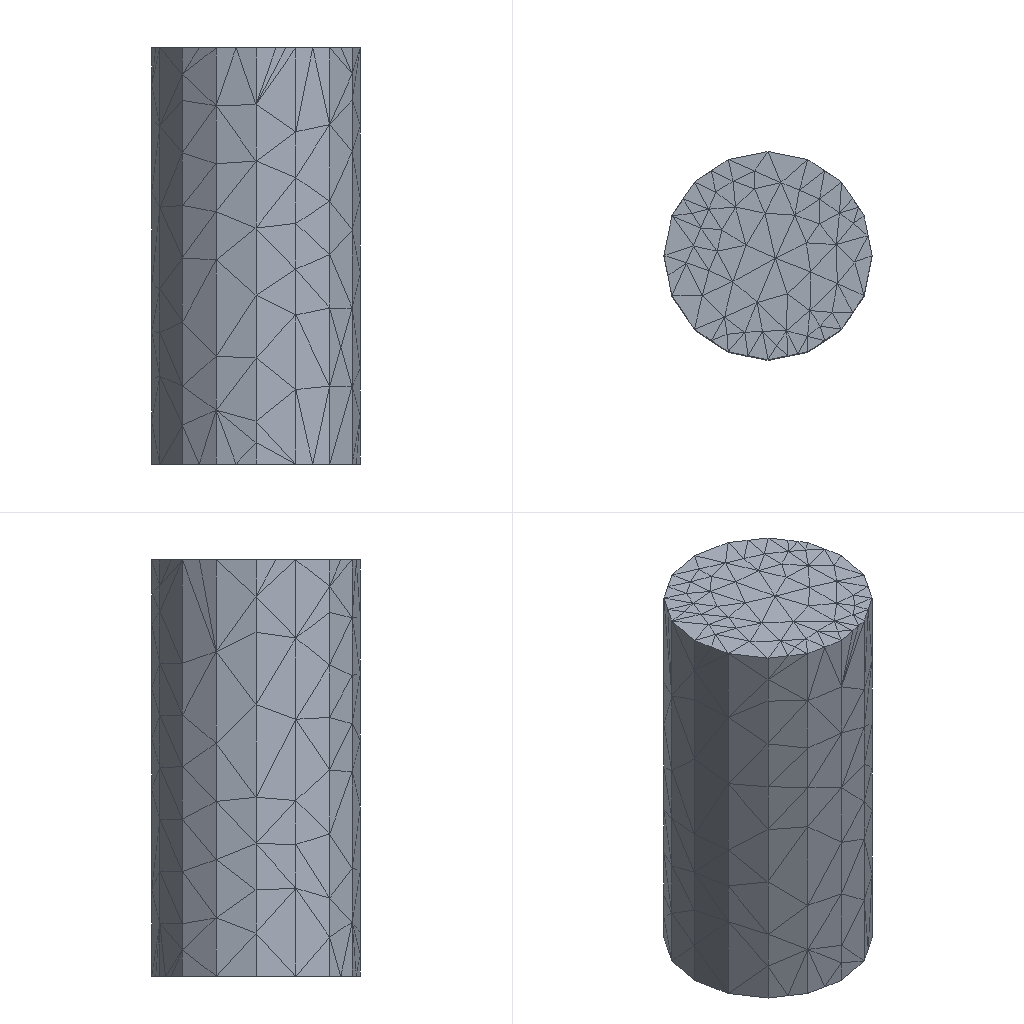Simulation study | ansys electronics desktop
Set-up summary:
category,name,step,type,value,unit,region
solver,ansys_electronics_desktop
units,length mm,,stated,model units
analysis,DESIGN_1,,HFSS Modal Network,design_type=HFSS
setup,Setup1,DESIGN_1,HfssDriven,frequency=10GHz; max_passes=6; max_delta_s=0.02
sweep,Sweep1,Setup1,Discrete,8GHz..12GHz n=9 step=
mesh,nodes,,,n/a (no mesh stored)
mesh,elements,,,n/a (no mesh stored)
material,vacuum,,permittivity,1
load,1,DESIGN_1,wave port,,,faces 8
load,2,DESIGN_1,wave port,,,faces 9
bc,PerfE,DESIGN_1,perfect e,,,faces 7
Ansys Electronics Desktop project file, long lists of numbers shortened, first 430 of 1282 lines:
$begin 'AnsoftProject'
	Created='Fri Sep  4 17:10:25 2026'
	Product='ElectronicsDesktop'
	FileOwnedByWorkbench=false
	$begin 'Desktop'
		Version(2026, 1)
		InfrastructureVersion(1, 0)
		$begin 'FactoryHeader'
			$begin 'geometry3deditor'
				KernelVersion(2, 0)
				ProjectContainsGeometry3D='1'
			$end 'geometry3deditor'
		$end 'FactoryHeader'
	$end 'Desktop'
	UsesAdvancedFeatures=false
	PreviewImageDesignId=1
	NextUniqueID=0
	MoveBackwards=false
	$begin 'HFSSEnvironment'
		Version(1, 0)
	$end 'HFSSEnvironment'
	$begin 'PlanarEMEnvironment'
		Version(1, 0)
	$end 'PlanarEMEnvironment'
	$begin 'Q3DEnvironment'
		Version(1, 0)
	$end 'Q3DEnvironment'
	$begin '2DExtractorEnvironment'
		Version(1, 0)
	$end '2DExtractorEnvironment'
	$begin 'NexximEnvironment'
		Version(1, 0)
	$end 'NexximEnvironment'
	$begin 'NexximNetlistEnvironment'
		Version(1, 0)
	$end 'NexximNetlistEnvironment'
	$begin 'EmitEnvironment'
		Version(1, 0)
	$end 'EmitEnvironment'
	$begin 'Maxwell3DEnvironment'
		Version(1, 0)
	$end 'Maxwell3DEnvironment'
	$begin 'Maxwell2DEnvironment'
		Version(1, 0)
	$end 'Maxwell2DEnvironment'
	$begin 'RMxprtEnvironment'
		Version(1, 0)
	$end 'RMxprtEnvironment'
	$begin 'MaxCirEnvironment'
		Version(1, 0)
	$end 'MaxCirEnvironment'
	$begin 'SimplorerEnvironment'
		Version(1, 0)
	$end 'SimplorerEnvironment'
	$begin 'IcepakEnvironment'
		Version(1, 0)
	$end 'IcepakEnvironment'
	$begin 'IcepakFEAEnvironment'
		Version(1, 0)
	$end 'IcepakFEAEnvironment'
	$begin 'SchematicEnvironment'
		Version(1, 0)
	$end 'SchematicEnvironment'
	$begin 'geometry3deditor'
		Version(1, 0)
	$end 'geometry3deditor'
	ReadVersion=12
	$begin 'DesignMgrEnvironment'
		CompInstCounter=1
		GPortCounter=0
		NetCounter=0
		Alias('Ieee;Simplorer Elements\\Ieee', 'Std;Simplorer Elements\\Std', 'Basic_VHDLAMS;Simplorer Elements\\Basic Elements VHDLAMS\\Basic Elements VHDLAMS', 'Digital_Elements;Simplorer Elements\\Digital Elements\\Digital Elements', 'Transformations;Simplorer Elements\\Tools\\Transformations\\Transformations', 'HEV_VHDLAMS;Simplorer Elements\\HEV VHDLAMS\\HEV VHDLAMS', 'automotive_vda;Simplorer Elem
	$end 'DesignMgrEnvironment'
	$begin 'ProjectDatasets'
		NextUniqueID=0
		MoveBackwards=false
		DatasetType='ProjectDatasetType'
		$begin 'DatasetDefinitions'
		$end 'DatasetDefinitions'
	$end 'ProjectDatasets'
	VariableOrders[0:]
	$begin 'Definitions'
		$begin 'Materials'
			$begin 'vacuum'
				CoordinateSystemType='Cartesian'
				BulkOrSurfaceType=1
				$begin 'PhysicsTypes'
					set('Electromagnetic')
				$end 'PhysicsTypes'
				$begin 'AttachedData'
					$begin 'MatAppearanceData'
						property_data='appearance_data'
						Red=230
						Green=230
						Blue=230
						Transparency=0.95
					$end 'MatAppearanceData'
				$end 'AttachedData'
				permittivity='1'
				ModTime=1499970477
				Library='Materials'
				LibLocation='SysLibrary'
				ModSinceLib=false
			$end 'vacuum'
		$end 'Materials'
		$begin 'SurfaceMaterials'
			$begin 'Steel-oxidised-surface'
				CoordinateSystemType='Cartesian'
				BulkOrSurfaceType=2
				$begin 'PhysicsTypes'
					set('Thermal')
				$end 'PhysicsTypes'
				surface_emissivity='0.8'
				ModTime=1461288057
				Library='SurfaceMaterials'
				LibLocation='SysLibrary'
				ModSinceLib=false
			$end 'Steel-oxidised-surface'
		$end 'SurfaceMaterials'
		$begin 'Scripts'
		$end 'Scripts'
		$begin 'AnsysComponents'
			NextUniqueID=0
			MoveBackwards=false
			$begin 'AnsysComponentDefinitions'
			$end 'AnsysComponentDefinitions'
		$end 'AnsysComponents'
		$begin 'Symbols'
			$begin 'DESIGN_1'
				ModTime=1788513025
				Library=''
				ModSinceLib=false
				LibLocation='Project'
				HighestLevel=1
				Normalize=true
				InitialLevels(0, 1)
				$begin 'Graphics'
					Rect(0, 0, 0, 0, 0.00254, 0.00254, 0.00508, 0.00508, 0, 0, 0)
					Rect(0, 1, 0, 0, 0.0004233, 0.00254, 0.0004233, 0.0004233, 0, 0, 0)
				$end 'Graphics'
			$end 'DESIGN_1'
		$end 'Symbols'
		$begin 'DefInfo'
			DESIGN_1(1002, 0, 0, 0, '', 1788513025, '', 'DESIGN_1', '', '', '', '', '', 'Design.bmp', '', 'Project', '', '', 1788513025, '', 0, 0)
		$end 'DefInfo'
		$begin 'Compdefs'
			$begin 'DESIGN_1'
				Library=''
				CircuitEnv=0
				Refbase='U'
				NumParts=1
				ModSinceLib=true
				$begin 'Properties'
					TextProp('Representation', 'SRD', '', 'DESIGN_1')
					TextProp('Owner', 'SRD', '', 'HFSS')
				$end 'Properties'
				CompExtID=6
				$begin 'Parameters'
					ButtonProp('CosimDefinition', 'D', '', 'Edit', 'Edit', 40501, ButtonPropClientData())
					MenuProp('CoSimulator', 'D', '', 'DefaultNetlist', 0)
				$end 'Parameters'
				$begin 'CosimDefinitions'
					$begin 'CosimDefinition'
						CosimulatorType=4
						CosimDefName='DefaultNetlist'
						IsDefinition=true
						Connect=true
						Data()
						GRef()
					$end 'CosimDefinition'
					DefaultCosim='DefaultNetlist'
				$end 'CosimDefinitions'
			$end 'DESIGN_1'
		$end 'Compdefs'
	$end 'Definitions'
	DesignIDServer=2
	MoveBackwards=false
	$begin 'HFSSModel'
		RepRewriteV2=true
		Name='DESIGN_1'
		DesignID=0
		'Use Advanced DC Extrapolation'=false
		'Use Power S'=false
		'Export FRTM After Simulation'=false
		'Export Rays After Simulation'=false
		'Export After Simulation'=false
		'Allow Material Override'=false
		'Calculate Lossy Dielectrics'=false
		'Perform Minimal validation'=false
		$begin 'TemperatureSettings'
			IncludeTemperatureDependence=false
			EnableFeedback=false
			Temperatures(6, '22cel')
		$end 'TemperatureSettings'
		ObjsEnabledForDeformation()
		'Port Validation Settings'='Standard'
		'Save Adaptive support files'=false
		SolutionType='HFSS Modal Network'
		$begin 'DrivenOptions'
			AutoOpen=false
		$end 'DrivenOptions'
		HasTransientSetups=false
		MaterialDensity=1
		MassOfTissue=1
		VoxelSize=1
		TissueObjectList=-1
		AverageSarMethod=0
		UseAutoDCThickness=true
		HaveZwaveSupport=true
		SolveInsideThreshold=100000
		RequireBodyFaceInfo=false
		$begin 'OutputVariable'
			NextUniqueID=0
			MoveBackwards=false
		$end 'OutputVariable'
		$begin 'ModelSetup'
			$begin 'DesignDatasets'
				NextUniqueID=0
				MoveBackwards=false
				DatasetType='DesignDatasetType'
				$begin 'DatasetDefinitions'
				$end 'DatasetDefinitions'
			$end 'DesignDatasets'
			VariableOrders[0:]
			$begin 'Editor3D Doc Preferences'
				BackgroundColorVersion=1
				'Plane Background'=0
				'Need Lights'=true
				'Ambient Light'=8355711
				'Num Lights'=1
				Light0[4: 16777215, 0.75, -0.15, -0.63]
				Ver=2
			$end 'Editor3D Doc Preferences'
			SnapMode=31
			WorkingCS=1
			$begin 'GeometryCore'
				BlockVersionID=3
				DataVersion=3
				NativeKernel='PARASOLID'
				NativeKernelVersionID=26
				Units='mm'
				ModelExtents=10000
				InstanceID=-1
				$begin 'ValidationOptions'
					EntityCheckLevel='Strict'
					IgnoreUnclassifiedObjects=false
					SkipIntersectionChecks=false
				$end 'ValidationOptions'
				ContainsGeomLinkUDM=false
				$begin 'GeometryOperations'
					BlockVersionID=2
					$begin 'AnsoftRangedIDServerManager'
						$begin 'AnsoftRangedIDServer'
							IDServerObjectTypeID=0
							IDServerRangeMin=0
							IDServerRangeMax=2146483647
							NextUniqueID=17
							MoveBackwards=false
						$end 'AnsoftRangedIDServer'
						$begin 'AnsoftRangedIDServer'
							IDServerObjectTypeID=1
							IDServerRangeMin=2146483648
							IDServerRangeMax=2146485547
							NextUniqueID=2146483654
							MoveBackwards=false
						$end 'AnsoftRangedIDServer'
					$end 'AnsoftRangedIDServerManager'
					StartBackGroundFaceID=2146483648
					$begin 'CoordinateSystems'
					$end 'CoordinateSystems'
					$begin 'OperandCSs'
					$end 'OperandCSs'
					$begin 'SubModelDefinitions'
					$end 'SubModelDefinitions'
					$begin 'Groups'
					$end 'Groups'
					$begin 'UserDefinedModels'
					$end 'UserDefinedModels'
					$begin 'OperandUserDefinedModels'
					$end 'OperandUserDefinedModels'
					$begin 'ToplevelParts'
						$begin 'GeometryPart'
							$begin 'Attributes'
								Name='CWG'
								Flags=''
								Color='(230 230 230)'
								Transparency=0.8
								PartCoordinateSystem=1
								UDMId=-1
								GroupId=-1
								MaterialValue='"vacuum"'
								SurfaceMaterialValue='""'
								SolveInside=true
								ShellElement=false
								ShellElementThickness='0mm'
								ReferenceTemperature='20cel'
								IsMaterialEditable=true
								IsSurfaceMaterialEditable=true
								UseMaterialAppearance=false
								IsLightweight=false
								IsAlwaysHidden=false
							$end 'Attributes'
							$begin 'PhysicsAttributes'
								SuppressedForPhysics='False'
								SuppressedForPhysicsEditable=true
							$end 'PhysicsAttributes'
							$begin 'Operations'
								$begin 'Operation'
									OperationType='Cylinder'
									ID=5
									ReferenceCoordSystemID=1
									$begin 'CylinderParameters'
										KernelVersion=24
										XCenter='0mm'
										YCenter='0mm'
										ZCenter='0mm'
										Radius='10mm'
										Height='40mm'
										WhichAxis='Z'
										NumSides='0'
									$end 'CylinderParameters'
									ParentPartID=6
									ReferenceUDMID=-1
									IsSuppressed=false
									$begin 'OperationIdentity'
										$begin 'Topology'
											NumLumps=1
											NumShells=1
											NumFaces=3
											NumWires=0
											NumLoops=4
											NumCoedges=4
											NumEdges=2
											NumVertices=0
										$end 'Topology'
										BodyID=6
										StartFaceID=7
										StartEdgeID=10
										StartVertexID=-1
										NumNewFaces=3
										NumNewEdges=2
										NumNewVertices=0
										FaceNameAndIDMap()
										EdgeNameAndIDMap()
										VertexNameAndIDMap()
									$end 'OperationIdentity'
								$end 'Operation'
							$end 'Operations'
							$begin 'SubregionDependencyInformation'
								ChildSubregions[0:]
							$end 'SubregionDependencyInformation'
						$end 'GeometryPart'
					$end 'ToplevelParts'
					$begin 'OperandParts'
					$end 'OperandParts'
					$begin 'Planes'
					$end 'Planes'
					$begin 'Points'
					$end 'Points'
					$begin 'GeometryEntityLists'
					$end 'GeometryEntityLists'
					$begin 'CachedNames'
						$begin 'allobjects'
							allobjects(-1)
						$end 'allobjects'
						$begin 'cwg'
							cwg(-1)
						$end 'cwg'
						$begin 'global'
							global(-1)
						$end 'global'
						$begin 'model'
							model(-1)
						$end 'model'
					$end 'CachedNames'
				$end 'GeometryOperations'
				$begin 'GeometryDependencies'
					$begin 'DependencyInformation'
						NumParents=1
						DependencyObject('GeometryBodyOperation', 5)
						DependencyObject('CoordinateSystem', 1)
					$end 'DependencyInformation'
				$end 'GeometryDependencies'
			$end 'GeometryCore'
			$begin 'AssignedEntities'
				AssignedObject[1: 6]
				$begin 'AssignedFace'
					kID=7
					$begin 'FaceData'
						ParentObjectID=6
						NormalValid=false
						$begin 'FaceGeomTopol'
							FaceTopol(2, 2, 2, 0)
							$begin 'FaceGeometry'
								Area=2513.274
								FcUVMid(-10, 1.22464679914735e-15, 20)
								$begin 'FcTolVts'
								$end 'FcTolVts'
							$end 'FaceGeometry'
						$end 'FaceGeomTopol'
					$end 'FaceData'
				$end 'AssignedFace'
				$begin 'AssignedFace'
					kID=8
					$begin 'FaceData'
						ParentObjectID=6
						NormalValid=false
						$begin 'FaceGeomTopol'
							FaceTopol(1, 1, 1, 0)
							$begin 'FaceGeometry'
								Area=314.159
								FcUVMid(0, 0, 0)
								$begin 'FcTolVts'
								$end 'FcTolVts'
							$end 'FaceGeometry'
						$end 'FaceGeomTopol'
					$end 'FaceData'
				$end 'AssignedFace'
				$begin 'AssignedFace'
					kID=9
					$begin 'FaceData'
						ParentObjectID=6
						NormalValid=false
						$begin 'FaceGeomTopol'
							FaceTopol(1, 1, 1, 0)
							$begin 'FaceGeometry'
								Area=314.159
								FcUVMid(0, 0, 40)
								$begin 'FcTolVts'
								$end 'FcTolVts'
Last 395 lines:
					UDirnZ='0'
					VDirnX='0'
					VDirnY='1'
					VDirnZ='0'
					WeightType=3
					EdgeTaperX_db='-200'
					CosineExp='1'
					DifferentialType=0
					Behavior='UseScanAngle'
					ScanAnglePhi='45deg'
					ScanAngleTheta='45deg'
					UDirnPhaseShift='0deg'
					VDirnPhaseShift='0deg'
				$end 'ParametricArray'
			$end 'ArraySetup'
			$begin 'NearFieldSetups'
				NextUniqueID=0
				MoveBackwards=false
			$end 'NearFieldSetups'
			RadFieldComputationVersion=1.8
			RadfieldHeaderFile='RAD6E9724520178851305017.tmp'
			RadPowerMethod=0
		$end 'RadField'
		$begin 'SolutionManager'
			$begin 'SimSetup'
				TypeName='BaseSetup'
				ID=6
				Name='Setup1'
				$begin 'Solution'
					ID=7
					Name='AdaptivePass'
					$begin 'SimDataExtractor'
						IsPortOnly=false
					$end 'SimDataExtractor'
				$end 'Solution'
				$begin 'Solution'
					ID=8
					Name='LastAdaptive'
					$begin 'SimDataExtractor'
						$begin 'Sweeps'
							$begin 'Sweep'
								Variable='Freq'
								Column='10GHz'
								Units='GHz'
							$end 'Sweep'
							$begin 'PostprocessSweep'
								Variable='NormalizedDistance'
								RegularSweep=1
								Units=''
								Minimum=0
								Maximum=1
								Increment=0.01
								CreateIndexedSubsweepFlag=false
							$end 'PostprocessSweep'
							$begin 'PostprocessSweep'
								Variable='Phi'
								RegularSweep=1
								Units='deg'
								Minimum=0
								Maximum=6.283
								Increment=0.08727
								CreateIndexedSubsweepFlag=false
							$end 'PostprocessSweep'
							$begin 'PostprocessSweep'
								Variable='Theta'
								RegularSweep=1
								Units='deg'
								Minimum=0
								Maximum=6.283
								Increment=0.08727
								CreateIndexedSubsweepFlag=false
							$end 'PostprocessSweep'
							$begin 'PostprocessSweep'
								Variable='Phase'
								RegularSweep=1
								Units='deg'
								Minimum=0
								Maximum=6.283
								Increment=0.08727
								CreateIndexedSubsweepFlag=false
							$end 'PostprocessSweep'
						$end 'Sweeps'
						IsPortOnly=false
					$end 'SimDataExtractor'
				$end 'Solution'
				$begin 'Solution'
					ID=14
					Name='Sweep1'
					$begin 'SimDataExtractor'
						IsPortOnly=false
					$end 'SimDataExtractor'
				$end 'Solution'
			$end 'SimSetup'
			$begin 'Version ID Map'
				V=1
				$begin 'Setup'
					N='Setup1'
					V=0
					Soln(N='AdaptivePass', V=0)
					Soln(N='LastAdaptive', V=12)
					Soln(N='Sweep1', V=0)
				$end 'Setup'
				IQM=0
			$end 'Version ID Map'
			$begin 'ID Map'
				$begin 'Setup'
					N='Setup1'
					I=6
					Soln(N='AdaptivePass', I=7)
					Soln(N='LastAdaptive', I=8)
					Soln(N='Sweep1', I=14)
				$end 'Setup'
			$end 'ID Map'
			ValidationCacheHeader=''
		$end 'SolutionManager'
		$begin 'UserDefinedSolutionMgr'
			NextUniqueID=1000000
			MoveBackwards=false
		$end 'UserDefinedSolutionMgr'
		$begin 'DatasetSolutionMgr'
			NextUniqueID=2000000
			MoveBackwards=false
		$end 'DatasetSolutionMgr'
		Notes=$begin_cdata$ $end_cdata$
		$begin 'AnimationSetups'
		$end 'AnimationSetups'
		CacheHeaderFile='HDR6E9724520178851305018.tmp'
	$end 'HFSSModel'
	$begin 'DataInstances'
		DesignEditor='TopLevel'
		Refdes('0', 'U1')
		$begin 'CompInstances'
			$begin 'Compinst'
				ID='0'
				Status='Status'
				CompName='DESIGN_1'
				GatesInUse()
				$begin 'Properties'
					TextProp('ID', 'SRID', '', '0')
				$end 'Properties'
				$begin 'Parameters'
					MenuProp('CoSimulator', 'OHD', '', 'DefaultNetlist', 0)
					ButtonProp('CosimDefinition', 'OHD', '', 'Edit', 'Edit', 40501, ButtonPropClientData())
				$end 'Parameters'
			$end 'Compinst'
		$end 'CompInstances'
		$begin 'Instance'
			DesignEditor='DESIGN_1'
			ID='0'
			$begin 'HfssDesignInstance'
				DesignInstanceID=1
				$begin 'WindowPosition'
					$begin 'EditorWindow'
						Circuit(Editor3d(View('View Orientation Gadget'=1, WindowPos(3, -1, -1, -8, -31, 208, 208, 1813, 671), OrientationMatrix(0.02598, -0.015, 0.02121, 0, 0.02598, 0.015, -0.02121, 0, 0, 0.03, 0.02121, 0, 0, -0.6, -6.073, 1, 0, -2.542, 2.542, -1, 1, 1.149
					$end 'EditorWindow'
				$end 'WindowPosition'
				$begin 'ReportSetup'
					$begin 'ReportManager'
						$begin 'Reports'
						$end 'Reports'
						NextUniqueID=0
						MoveBackwards=false
						$begin 'NextVersID'
							NextUniqueID=0
							MoveBackwards=false
						$end 'NextVersID'
					$end 'ReportManager'
					$begin 'Reports'
					$end 'Reports'
					$begin 'ReportsWindowInfoList'
					$end 'ReportsWindowInfoList'
				$end 'ReportSetup'
				$begin 'Properties'
				$end 'Properties'
				$begin 'UserDefinedDocument'
					$begin 'Data'
					$end 'Data'
				$end 'UserDefinedDocument'
			$end 'HfssDesignInstance'
		$end 'Instance'
		$begin 'SODInfo'
			$begin 'DESIGN_1'
				$begin 'CosimDefinition'
					CosimDefName='DefaultNetlist'
					$begin 'SODInstanceMap'
					$end 'SODInstanceMap'
					SODComponentList()
				$end 'CosimDefinition'
			$end 'DESIGN_1'
		$end 'SODInfo'
	$end 'DataInstances'
	$begin 'WBSystemIDToDesignInstanceIDMap'
	$end 'WBSystemIDToDesignInstanceIDMap'
	$begin 'WBSysIDSysDetails'
	$end 'WBSysIDSysDetails'
	$begin 'WBConnIDConnDetails'
	$end 'WBConnIDConnDetails'
	$begin 'WBMaterialGuidDetails'
		WBMaterialGuidMap()
	$end 'WBMaterialGuidDetails'
	$begin 'MinervaProjectSettingsBlk'
		MinervaRemoteFilePath=''
		FolderContainerString=''
	$end 'MinervaProjectSettingsBlk'
$end 'AnsoftProject'
$begin 'AllReferencedFilesForProject'
$end 'AllReferencedFilesForProject'
$begin 'ProjectPreview'
	ProductName='ElectronicsDesktop'
	MajorVersion=2026
	MinorVersion=1
	IsEncrypted=false
	Thumbnail64='/9j/4AAQSkZJRgABAQAAAQABAAD/2wBDAAEBAQEBAQEBAQEBAQEBAQEBAQEBAQEBAQEBAQEBAQEBAQE\
BAQICAQECAQEBAgICAgICAgICAQICAgICAgICAgL/2wBDAQEBAQEBAQEBAQECAQEBAgICAgICAgICAg\
ICAgICAgICAgICAgICAgICAgICAgICAgICAgICAgICAgICAgICAgL/wAARCABgAGADASIAAhEBAxEB/\
8QAHwAAAQUBAQEBAQEAAAAAAAAAAAECAwQFBgcICQoL/8QAtRAAAgEDAwIEAwUFBAQAAAF9AQIDAAQR\
BRIhMUEGE1FhByJxFDKBkaEII0KxwRVS0fAkM2JyggkKFhcYGRolJicoKSo0NTY3ODk6Q0RFRkdISUp\
TVFVWV1hZWmNkZWZnaGlqc3R1dnd4eXqDhIWGh4iJipKTlJWWl5iZmqKjpKWmp6ipqrKztLW2t7i5us\
LDxMXGx8jJytLT1NXW19jZ2uHi4+Tl5ufo6erx8vP09fb3+Pn6/8QAHwEAAwEBAQEBAQEBAQAAAAAAA\
AECAwQFBgcICQoL/8QAtREAAgECBAQDBAcFBAQAAQJ3AAECAxEEBSExBhJBUQdhcRMiMoEIFEKRobHB\
CSMzUvAVYnLRChYkNOEl8RcYGRomJygpKjU2Nzg5OkNERUZHSElKU1RVVldYWVpjZGVmZ2hpanN0dXZ\
3eHl6goOEhYaHiImKkpOUlZaXmJmaoqOkpaanqKmqsrO0tba3uLm6wsPExcbHyMnK0tPU1dbX2Nna4u\
Pk5ebn6Onq8vP09fb3+Pn6/9oADAMBAAIRAxEAPwD+rnTfH/7fXxx/aA/bO8I/BT43fsgfB/4Zfsz/A\
LQHgn4F+GdH+KX7HPxo+OvjvxF/bf7IH7LP7SGs+Kdd8b+E/wBvL4e6fHu8QftB6rp1rY2/hyP7PZ+H\
Ld5by6nmkZfQP+Fc/wDBU3/o8j9gD/xWn+0V/wDTYq/Er/goPrX7Z3hTV/2tvHv7EOj/ALQnif4g/C7\
/AILq/Ar4wfEHwV+zvbfETUNY+I3wl+D/APwQr/Zp+J+q/C34h6P8Oo3l8RfDLxT448J+APDtxpWpRz\
aZqur+JtG05oZr+6sIn8I+Cn7Qv/BZf9k74Jfs6eDPFp/aP8YRfDf9nj/gpV4n+OPxJ/ap+HWu6n4Iu\
/G3w21f/gqj4z+BHjX42/tL/Fbw1d3nh3RftvwR/ZEi02bV/FvgvQ7Hwn8RdINpB41sPFtnc+AwD+iz\
/hXP/BU3/o8j9gD/AMVp/tFf/TYqP+Fc/wDBU3/o8j9gD/xWn+0V/wDTYq8t/wCCVXx5+K3x18K/tbD\
4n/FL4s/F2y+FP7Vmi/DX4ZeKvjn8EvCX7PnxWT4f3v7GX7H/AMWbjT/GPwz8I/D7wwmk6gfiP8U/iH\
dq15pMN6YdViiZYbWG1tLb5v8A+Ca+k/GWy/bC/a98RfG34n/tOX2oz/Fz9vKPQ/hr8afgj/wVO8PfD\
nwx8L4f24/E5+COu+Bfj18ev2htR/Zp8Y+HG+CNn4Hk8Mad8Nvh1oHiCHwxrkMdtq81npPi6XWgD7i/\
4Vz/AMFTf+jyP2AP/Faf7RX/ANNio/4Vz/wVN/6PI/YA/wDFaf7RX/02Kv8APS+EuqftaXnhTwt+33q\
kX7SnxA+InwL8SfA+81r9oLxdffEz4weD4/FXww0jwPpPjeX4n/HXx/rmp3eneL7vxz4t+EzaR4eubx\
re60vxZrVtplva6RoKWcf7pfCj/gpF/wAFK/2M/gZ8F/2kvj14++NP7Q37PFpqPg3wl4b8D/GT4ceC/\
h1/wuzwh49+I/8AwVN+Gvgm40/9o+4+Ds/iLxH4h0n4Tfsm/sY/EFdYu7rXtV1/TvjlPqWv3Wo23i/Q\
NXtAD93P2sfFv/BU39l/9lj9pb9pf/hqD9gDxx/wzv8As/8Axk+On/CFf8O7v2ivDP8AwmH/AAqT4de\
I/H//AAi3/CR/8PS9Q/4R/wDtD/hH/sn277BffZPtfn/Y7ny/Jf8AX6v4pfjT/wAFLfi34D/4JRftIf\
Bbxf8AsxftDeNPgD+03pv/AAVT/Zp/Zz/au+L37Qmp/Ev4kSXPjT4tftXeDPhV8L/iloXxRvta8XWet\
eCdGudJ8H3z+J/FE+py2/wtvrjTm1O3tY9/6+ftS/8ABYTx/wDAD9tD4kfshfCn9myP9qXxj4U8M+GP\
FA8OaR40sPglq3he2v8AwP4f8WXmlf8ACSeI5fEMfxc8SagnibTJLDT9N0XQbqD7Ta6baR+Ir+7Y2sz\
nClCVSpONOENW5NRS+baRyYzHYPL6ca2OxEcJQlJQ9pUfLTjJpuPPUfuU1JrljKbjGU3Gmm5zhGX7vU\
V+IHjz/gsH498D/sTeIf2vtR/YQ+MWg3fgL4i+CPCnjvwB8RPEV94G8M3HgXx8l7a6B8X/AIR/GSP4b\
ajpXxm8Dza+/huxin021ggl/wCEiivPtK2cmny6l9Bfto/8FLNB/Zj+H37KHif4W/DL/hofxf8Atl+O\
vBvhb4K+BYPHS/Dw67ofjLRtN1K08WLrqeENeMkEd74n8DWpt0sjvPitJTcIIdktHWfp7RX4r+L/APg\
rR8SPFX7RHx8/Z7/Yx/Yg8Yftcal+zBqU2h/GnxEnxu+H/wAGotI1uxv9U0jVrDwloPirSL688a/Ztb\
0TWLDFusVxNd6ZIkNs8MlrPcfpB+y18e9R/aS+D2h/E7W/gv8AGL9n7xBeXd9pXiD4WfHHwRr3gbxr4\
e1fTWiFwYrTXtNtW13w9NHPBLZanbxCC5jkKOkF3BdWtuAfjP4j+PXxX/Z3/av/AG79S0z9rv8AZb/Z\
t8BfHr/gqt+zh+y98OtF+OP7EX7Qf7TviPxr+0t8Tf8Agl5+wLfeFNGtfG/wa/a/8CWXgjw1qOg6AI0\
bWtDTTtNn0C7u9R8TrFqFpZ2e54J/bx8UfG74O/D74l23/BYH/gjxb/Cv9oDw/wDEOf4f2vxq/YD+OH\
wZ1D4leFPAvinxf8NviPcWnw0+O3/BWDQda1Hw5Z+I/BfjGwvZLjSRayRaRPKDLZskz/Gn7dXwr+Gv7\
UnxR/b5+AHiX4g/tSfCDxn8Mf8Agqn8Kf2ofCHxF+B3/BOD9s/9t3w5a67Z/wDBFX9lf4L+C4LrX/2d\
fhzeaHoHiXS/F/xDtfEb6fda4mqiDwhaRTada2uvWOrReGX37IHgix+A3wC/Zw8C/tc/8FEPDXwl/Z8\
8eN8VPDHgDVf+CEf/AAVv1r4ear8RbH9vHx9+2homueJvh5ong3RtK8b6b/YnjLRvBmoad4nt/ENsw8\
Bab4j0H/hG7ubUtPvgD9B/En7HvhPxd8KU0YeI/wDghH8d/hp+z9peueO9E+Fnwn/4IWeN/wBpq8+HG\
nfEzxx4h8CeJfEXw/8Agb8H/wDgoz4k1a0l8QfET4J+L9Kv5NC0R5tV1b4Oata3AnufDd8tj80/tu/8\
FUPjh4e/Za+KDeFf23/2bPi9d+OfBk/gP+xfhh/wST/b0+Dl9pF78QNZ8Y/DXXfCuuftBfED9s/xB4T\
/AGfPjfpVt4R+JV4vhrxdp7eJ4JvA8qv4aPmROfr/AOBnxd8I/s9/sY+E/wBjf4f/ABB/bKj0T4U/CP\
4f/C34S+OdV/4IHf8ABTXVtRW38D+N/FF7qMPxm8Jah8AJdH+KfhHxF8J/+Fd+FdfsdNtvCms3E1h4u\
8R2XiWw1LxRo8fgz4T8C/AD4c/BAafrn7NvxY/aC+BvxQ8O6p488X+Cfi54Y/4Nnf8AgopB478Ha/8A\
FHSPFvhjxX8JbbW/D/wj0q68XfsZ6VoHjbUJvA/w28TXOuan4S1fwX4KmHjnVNB8G6R4bAB8Y/sgfsI\
6D+0N8JfBf7Onw6/4K8fGDwdqHxjs9U0/xf8AswaN+z1+0mn7POlfHmw8BXHxO+IX7OvjX4jN8Q9L8B\
ah8dtF8N+Fr+/13wzdIniiCw8Kz6q+hPZWqTH4u+Mn7THxk8cf8Exvh/8AssfErxz4e+y/sv8A7Vlt4\
Qi+ETfs0fGSw+JvhKK28F/F650LXfiJ+1Fc/E+58F6dbfb9f8e6BpHgO88H6H4pvYfBF1qOn399YeF9\
eA/eP4IeAPhv8GPjPo/7Q+n+LvjsfjJ4csPHGqaP4x8Of8G7v/BYzSNVn8YeIPgj4l+C+g+DvFHizxb\
J4i8VeLf2VTq+r6f8S/FfgC78SnWPF3xgXVvHz+PdIudZaws9C/g0vwz4u1z4+eFfFP7TPxJ/aDufjH\
8Gvi1f2PiP/ghf/wAFUvgJ8MfjZqPwD+FP7Sfw5+HXiX4+r8K/2XNZ/tD47TeIf2gfDfiLxT400LRNN\
sPEEf7Pvhbw1pvg7wtaKmqaeAfDn/BViXxTD/wTp+G3hLwR4/8A2VdS/Zd+HP7V3hjRvAngn9mH/glx\
+0h+wJ8Oj4m8V+AP2gvFT+Nfg/48+Kf7Snirwd8Yvhfezy+NLq7uvA2j3mn6lqfie31f/hJUy8Gq+xf\
8FtfAH7JN1+2b4m8RfFnTP2hPgV8R7vRPBV/Z/tF+EvDbav8ACfxeNM8E+HrDTtOkl0S41K/fxbYRww\
2xWOx0mVItPBnuJIGsZJfhHW/2ufhL+xp/wTy/4KYfBL4aeDdc8d+FvHfwL+Fn7BOgfETwv+zR8ff2a\
vhp4u0rQv2e/jlofxb+I3xO0v4o+EZH8NftrWOl+ML7QtZTxTeaXrfiux8A+F72w8PT6H4U1Rk+3fjT\
8dP2gv2lviZ+0VqnxJ1z4HeGdO+APxg+Kfwj+LTa9YeM3+FGmT/A2w0/whN408J+CTrzahfPqd/Yw3z\
WOpeJRYWJ8qY2+p39payN/O/0lM6xfDfB/DOfUM4r5JhMsz3DSxdXC46pgcXPD1cBmWGjQwtsFmGHxl\
eriq2GjTy/GYSth8XL3IxeKWGPzDxXzbEZXkWU0sLQr1K2dZlh8AqmGxEMNVw/1qliI+3VSrhcZRlyt\
KCpVsPUp1pVFTlF81n9k/8ABIjwr+0J+2V/wT6/a4/Zr/aL1Xxd4v8A2cNX0+9+EX7KHxV+JGgXumeJ\
tV8LXWleKbI6lpy6oXutR8M+HdUs/h/e6MZZLyPT7k3OjW11JbaVHaWfxf8A8EevD/xh/ax/bP8AgL4\
T+Ouiz2/hv/gkd8HPHHw9Gn3zyXcR+K+o/Efxn4d8IW2owugGn6rYaM0FvbqhKj/hRtrMSWkaNfsf4n\
f8FHvjP8Mf+CIXwX+Mnwotb34dftGeOfCserWF5p2maLrQ+HXw58IftD6P8OfEXxPu9J8c6Tf2uoeHt\
Wl17wTo9os9vLK8nxZtry0JFnJPD7B4r+H+p/8ABE34D/DPUPh18WPAXjn4p/tmft+fC7wH+0v+0/8A\
tO+FtRm8N6Zo/wAT9H+Imoa78R77w74d+Kvh7+zNN0CbRrnVZBqHiZ4W/tbWpbu+iW6hlsP3jKauLr5\
VllbMKEsLj62Hoyr0pzp1J060qcXUpynSjClOUJuUZTpQhTk03CMYtJfoOWVMTWy3L62Noyw+Mq0KUq\
1OUoTlTqypxdSEp0owpzlGbcXKnCMJNNwjGLSXwj/wUW+HH/BOTQP2wPjL438UeMv25f8AgnH+1FZah\
eeKdH+L3hf4danrvwl+OvirUkeY+L/hVN8NdY1HUZNR1G4W3muZ/wC1PCtubm9mW/ih1T7csX7Yf8EZ\
fiZ+1v8AFr9iDwt4v/bHtvELfECbxf4jsfBGveMdH/sLxl4w+E9pZaEfC/ifxRYvawSTX8urTeJbeC8\
mgjm1HT9MstQka5a6+2XGL+zr+3z8bvido37Yz6X8PPBX7Wyfs9ePPhH4J+C3xN/ZXs7zwZ8Mv2lb/w\
CKVtpdvrFpoFz41+Ifiiy0C28HazqcDeK9Vh8R6rZWWmrPexxSG2WK5+i/+Ca37UXjb9s/9ir4N/tLf\
EXQ/Cvhrxf8Spvia2p6H4Kt9XtfDen2/hD4v+P/AAHo0VjFrur3900zaH4X017qSS5ZZbuWeWKO3heO\
3i9A7j83fjH+3n/w7v1X/gpt8av+FVf8Lf8A+Eo/4Ks/Bv4Xf8I1/wAJz/wr/wCw/wBtf8Egf2D/ABZ\
/bv8AbP8Awh+t/afK/wCEJ+z/AGX7JHv/ALT837Qnk+XL8ff8RRP/AFY3/wCbMf8A5P1eZ/8ABY//AJ\
I//wAFC/8AtNl+z9/65R/ZKr+X+v5N8X/EzjfhbjOvlORZ39Ry+GHw81T+rYSraU4tyfPWw9Ser6c1l\
0SP+gz9nL9B/wCi948fRpyzxA8V/DD/AFq4uxGcZthZ4v8AtriHA3oYarTjQp/V8tzbB4VckZNcyoqc\
r3nKTsf6GX/BLv8A4Kif8PJv+F5f8WN/4Ux/wpj/AIVn/wA1M/4WL/wkn/Cxf+Fg/wDVPtC/sf7H/wA\
IJ/09faP7V/5YeR++97/4KKi5uf2atc0iwi/aLsNW1/WItI0Dx1+zVpH7TvinxT8LfEsnh/xHd+GPHn\
jTwN+xt8XPBvxJ8efDVPEFnpmmX+meGtQvC134m0671ewTQbTVNU0z8Hv+DXb/AJvk/wC7Z/8A34Gv6\
d/jL8ZvBfwG8D3nxE+IFp8RLvwxp91Ba3x+GPwb+MHxz8RWgnjnmN/ceCfgh4F8Ra1FokMNtM91qDae\
LGzQBru4hV0LfuPhZnmacR8B5FnWdYr65mWM+te1q8lOnzezxmIpQ9ylCnTVqdOEfdgr2u7ybb/yy+n\
p4XcCeC/0sPFbw08NMi/1a4J4a/sL6lgvrWMxnsfrnDeT5hif9pzDEYrF1PaYvFYit+9xFTk9p7Ony0\
owhH+RT4Rz/wDBSyyu/gJbftu6F/wUcvtB1LxN4r/4bl1f4B3P/BR8fFX4X+CvDXgH4l6d+y94V8B6l\
+z14+k8FfG298U+KdX+Dep+LNa+CngrQtR8O3Hwy1W1+JN/fQeKb22tvoz/AIJ7fDX/AIKO/GbwPbfC\
r41/Fn9t74IftJeOf2Sf2mvC37YHxT+Onhb9pDxP8FvCXxX1L9o74Dw/sran+zppPxE8SaN4LfxVP+y\
kPjRaatP8NdUtptP1W+XUPEch162iSX9oNH/4Kx/8E+9f8I/Er4g6R+0LZXvgD4UfB7xb8fPE/jtPhz\
8Xo/BerfCT4f3Wh6b4/wDF/wAM/Fc3w/Ww+NMega74n8N6Vrln4OuNe1HR9a1+y0TUbS21a6hsn94+G\
f7Y37PHxf8AjJ45+AXw/wDGusav8UPh4PGza/pWofDb4peF/D2op8M/GWnfDv4lP4F+IXivwVY+HPih\
H4c8favpmia+3hnVtXGi6rfR6fqRtbpvKr9BP5APxe/4KOf8E39L0T/gjL+1n8HvHmv/AAdj+Hv7M3w\
S+In7S3wh0X9nv4G+LfgpMviv4L/CH4o634og+IWp+P8A9oD4hz+O9Q8T6JeXNhLqpexvrKa8n1C5bV\
3eKCD5K/ao/wCCempeC/EPxC8PSfGDRfGOp6l8bPF37RnxvbxX8Ktbl8E/GLx78Q9L07x6mn6h4R8Pf\
FvTX8OeDLHXLqeS00qTVdWF2+nwSX00qWgiuf3z/wCCsX/KLL/gpZ/2YB+2R/6zr8Rq/Nr/AIKI+M4o\
Pj58TPDduksc0Uvgx76aYReROv8AwgHhW+tLW3UFnfdNJC7t+6ZPsxUb0diP4r+nNmXF+V+G/AFfgnG\
ywOdVeMMup86o0a69lLK86bvSxFOrTcoVI06tGah7WhiadHEUJ061KnUj+H/SD43yvw88OsZxTmVanR\
rYCsngnUp06jeOWHxM8P7NVYVIQqRcJVFVcW6UYSqK7jZ90v8AwTQ8Lftwf8E9vCnhnxZ4/wBc+G3xr\
8Y/D7SvA7/FHwdB8WPDfw6i8HeCv2j/ABL8V9E0fVf2YNN+PEHhjxtpyrqGsw6fdavLdTQy6tba5ZfZ\
Gs9OsLP9E/2m/wBjWy/aD8P/ALInhrTfiHrHg3Tv2Tv2p/gF+0jYXHiK31/4ra/47svgTZa/YWvgjXP\
FfizxrHqkusapBrUbXXiXUrzWdQaa1e5vLfUbi5klHd/sZWbWH7L3wYs38zfB4SCP5k0877zqeoM3zX\
JLRruY7YvuQriKMCNFA+nK/rLg/Kf7A4S4XyLkjT/sXLsFhOWFONKMfq2GpUeWNKDcKcVyWVOLcYK0Y\
uyR934a1K1bw54ArYmUZYirkmVSqOCtBzlgaDm4pwpNRcm+Vezp2Vvch8K+OfgP+yaf2efjv+0N8Qvh\
/wCO7fT/AILfH/UND8cTfs923g82ej+AvjFb2kVh4z+IfhLxPD4oMVra+JYYo7jV9LXRYw+oQRXcV6i\
q8Es/7BX7KX/DEP7J3wp/Zf8A+E9/4Wd/wrH/AITn/iuP+EW/4Qv+2/8AhNPiT4x+IX/Is/8ACRat/Z\
v2b/hLPsf/ACELjzv7P+0fuvN8iP6/or6I+1P5l/2y/Dnh7xPpn/BSew8S6Do3iGxh/wCCu/wRvIrLX\
NLsdWtIruP/AII4/sRwx3UdtfwSIlwsNxOgcKGCzuoOGYH8pP8AhUXwn/6Jh8PP/CK8N/8Aysr9pvjx\
4A8XfEe9/wCCmeh+DNJ/tnVLX/gq/wDBrVZ7X7fpmneXYQf8Efv2E7OWfz9VvYI2xcX1quxXLnzchSq\
sR8Qf8MrfHr/oRP8Ay6PBn/zRV/h19PTjbLci+kFmOAxPF1DJqscqyyfsKmPp4eSUqU2pezlVg0pWun\
y623P9p/oOeImU8NeA2X5XjOOsPkFaGZ5lP6vVzOlhZJTqQan7GVem0pWupcvvWvdn6N/8ES/CHhPwr\
/w0z/wi/hjw74b+3/8ACmft39g6Lpuj/bfsv/C1/s32v+z7aP7R5f2i48vfu2ee+3G5s/qX+1h8D/F/\
7Q3wi1D4X+E/Gnw68K2+u3zW3jPQ/jJ8DNF/aL+D3xO8C6joeuaFr/w6+Jnwu1PxZ4eutW8PTnWLTUr\
ebSvEWiX1vq3hfTXnub3SDqmi6p8L/wDBKX4VePfhl/wvr/hN9B/sT+2/+FXf2Z/xNNG1L7V/Zv8Aws\
X7b/yCNRuPJ2fb7T/WbN3m/Ju2tt9u/wCCm37QOi/s2/s6af4+179ri2/Y3tNQ+I+g+E7Px9DoPwZ1T\
xX471/WfDvi6fwx8I/Auu/tErP4G+Hev6t4j07Srq88ReKrC/0bTdA8N619rOjrMPEmif6QfQszSjnP\
0Z/DXMsPmMc1o4n+2eXEQrKvGpycQZrTdqsZTUuRwcHaT5XFx0asv88vpi5zh+IPpHeIub4XNYZ3Qxf\
9kcuKp144mFX2eQ5XSdq0ZTjPkcHTdpPlcHDRxsvg/wAdf8EVvi38Yv2Zvj5+yR8af239O8a/DHx9+z\
F4R/Zh+BfxB0z9nLWdC/aL+Bvgv4Va/wDDDxD8M9I134han+0jqvhr4neDr/UfhjZT/Eu1s/BHhTxF8\
RLjUo2l8XaDbaN4dtNJ+x/2Tv8Agn348/Zx+Ndv8SvGn7S7/HTwz4L8P/tcaJ8KdP1z4N6D4E+KFtff\
twftIeAP2pv2g/FXxh+IHg3xdH4d+IniC++Kfw902XTI/DfgTwHpOlWmo3VrDpckX2cQfzrR/wDBTz/\
golPr3hHRNU/b8+AdzY+L9U+Idh48+JXgvxl+y54J+BfwysvAN5fWngTxt4q+Kfij9kDxvD+xR8KfiN\
Da2F/8LNd8X2/x8Hx40fX9N1Hw1B8IV1RI9O/TH/gkJ+3Z+0Z+1F8V/Auj/GX9oi/+JnirxV8Av2pvG\
v7Qf7O+t/C/4QfC3X/2SfGvwm/aQ+C3w2/ZkGs+CfBfh3/hKfh1qHxL+CHjDxt4sn0Xxj4k8RsZ9Ikf\
QrtNOtWB/qU/mU/TL/grF/yiy/4KWf8AZgH7ZH/rOvxGr8p/2+ILGD9sP4sahqDsSZfh/FZoVM0SzSf\
DPwRBZo8QZCm+/cKWDnYsxkVS64r9WP8AgrF/yiy/4KWf9mAftkf+s6/Eavx//wCCj8E2pfthfEzSIH\
ZRPH4KnkwkSGOf/hWnghLKeK5lhYxSosd637o7sLiQMjqj+3w3wlw5xdxBk9LifBxxuX5FWWZRhUipU\
1Vw8JwjKd/hShWqcskm+dxS5W1KP+e/7SOtQoeC/AlXGU1Xy+lxpls8TSlOdOFbD0soz6rVozqU7ThG\
rGHJzQalFyTi1KzP3s/Y/wAD9mv4TKLR7EpoF0klvIiIyzR65qqTyZTiRZJleRZB/rFlEh5avpOvmP8\
AY0Of2YvhCpvIb94fD15bTXMLK5a4tde1a3uYrmRbiUS6jFcRSRXT7gXuYZWKREmJPpyvPzDEUsXj8b\
iqE1UoYmtVqQlF8ylCc5Si1K7ummmnd3Wt3uf2/wADZtRz7gng/PMND2eHzrKsvxdOPNTnywxOEo1oR\
56MpUZ2jNLmpSlTlvCTi02UUUVyH1J+O3hH/kp3/BUv/tJb8Kv/AF0z/wAE8q2a5fQbqS0+JH/BUmSN\
UZm/4KZfChCHDEYP/BJb/gnqxI2sOcqKP7bu/wDnnb/98Sf/AB2v+X79qxhatb6XGcTgly/2Fki1f/T\
iofqfCXjdwJwJk8OH+IMRiaeY06lSq1Sw0qsOSq04+8pJXstV0PuD9lj/AJnv/uWP/dhr3T4p/F/4Tf\
Azwde/ET42fFD4d/B74f6bc2NlqPjn4p+NvDXw+8HWF5qdylnptpe+JvFup2lla3NxdyRxQRyTq8sjh\
IwzECvnf9ka9lvP+Fg+asa+X/wie3ywwzv/AOElznc5/uil/bk+HHx9+Jnwk0LSf2aPBP7O3i34raZ4\
+0/UbDWP2ifEeqeD7b4b+HdR8K+MfCPjHx78H/FmmfAr4ijw18cl8L+KNU0fRb678MXunW1r4v1OXUI\
dQtFl0XVf9mP2alOVL6FHgtCfxR/1jv8APi3Pn+p8VxPxRlXGeeY7iXJJzqZXmXsvZOpB05v2NGnh58\
0G21+8pTS11Vn1NXxD+37+wj4R8QeLPCfiz9tf9knwx4q8B6Do3irxz4a8Q/tH/BzRfEHgzwv4jPhdf\
D3iTxZo2peMornw7oN+3jfwWLK8vI4be6Pi/SxBJJ/aFp5vp/w//aP/AGePix4y8VfDr4WfHn4MfEv4\
g+BLOx1Hxv4F+H/xR8D+MvGXg3T9US3l0y+8VeGPDuu3N74es7iO8tGglu4IUmW6jMbMHXP4Q+Ff+CZ\
v7bPwQ0DTNM/Zq+FH7E/w+0fSINZtLH4WeJf2xf2vPip8O/Dd/wCNLfStGsfip8Gk+PX7NnjrT/2ff2\
g/h38IV8ffDfRfEvh/wzLo/wAQdN+LN94j8Q+E/C+l6PpPw2H0l/wTj/4J6fG/9k/4h/DWTxn4P/Z2+\
G3we+A/wl/bG+Hnwm8NfBj4v/E34seJLyx/bK/ag+En7TA8F+Lrzx98CPB6r4b+Glv8NX8HeG9V+06j\
feI9Nul1a703w1NLNpS/3SeCfWn/AAVi/wCUWX/BSz/swD9sj/1nX4jV+Uv7f8UUP7XPxeuojFPqEj/\
DtI7eZiwWD/hWng4vvRZUeGxCwSl2Qk+bLGvJcFP1a/4Kxf8AKLL/AIKWf9mAftkf+s6/Eavz5/ai8D\
2niX9t/wCLk2oCMWgh8E3Be7hY2RGnfC3wPNcK0nmKsnlRbJZI2JRw8aSKqtuP89fSe8Z818D/AAozL\
iLIcPPEZ3xFXp5JhI0oVKtZYjG0q9Wm6NKlGU6tW+FtCmrOTdovn5U/4j+nd4d5n4peG3hxwfllSVF5\
hxtlCrzjypww0sBnFGrJ819F7WPwxnUvb2dOpO0Jfrj+x60zfsz/AAgFxHLHMnhhoZPOeKR5TBquowi\
5DxSuGjlCCVNxEmyZfNSOTfGv0pXyH+whNrE/7K3wzk1kX5X7Z8Ro/Dk2o20FvNfeAIfin43i+GeqW8\
ltY28Wp6Xd/DtPC9zZahFF5ep2d3BqMckyXQmk+vK/YuD1iI8JcLRxeJljcWsuwKq1pwdOdap9Wpc9W\
cHCm4SqSvOUHTpuLbThBrlX9d8I5XLI+FOGMlm+aWT5dgsK33eHw1Kk3st3DsvRBRRRX0Z9Cfi9pf8A\
yUT/AIKkf9pNfhP/AOulP+Ce9UK8o+L3/IX/AOCm/wD2lX+Dn/roL9g6vkav+cX9plwf/bP0o82x39o\
/VubJcnjy+x5/ho1Ffm9rDftbQ/zs+kp9Iz/iGnifiuF/9Tv7a9lgsHW9v/aH1a/toSfL7L6jXty2tz\
e0d+yP3o/Y7/5qL/3KP/uz16T+1R8YfiT8DPhRe/EL4ZfC7wf8T7/SLy4ufE7fEj406P8AAL4Z/D7wP\
pHh3xB4l8SfET4g/Ee/8KeIbzTvD9rDoUFhFDpHh3XL+bUvElh51rZ6Qmqaxpnxd/wTA/5rh/3TT/3o\
FfcH7R/7MHwe/aw8FaD8P/jXp3jnUfDfhjx54a+Jmgn4e/GT4zfAzxFpvjjwd9ufwvrkHjX4F+P/AA3\
rTNY3d/JdQW76g1ot9a2l/wCQbyxsp7f/AFr/AGe2Xf2T9EDwiy/231j6v/b/AL/LyX5+KM6n8PNK1u\
a3xO9r6Xsf1f8AR/4z/wCIg+EfCXF/9m/2R/a/1/8A2f231j2f1fM8bhf43sqPPz+x5/4UeXm5fe5eZ\
/mj8Uv+Cv2ufDfUdP8AB17+yF8Q9B+Jvi74WfsS+Ovh94I+IGteMW1LVvE/7Xfw5/bI+KWv+B/FPhj9\
nv4MfEvxl4dn8EaD+xX8TdMv207wdr2sap4iV7OHw/ZaPBD4gvvWf2J/+ClGqftf/ETwloifCPwHoPw\
o+L/w/wD2oPiB8AfjH8PPjnqvxW0/4maV+x5+0D8OP2a/jLe6h4d1X4J+Fj4T0C68f/EvRb3wjepfan\
LrugAahfWWhXTtpsX0p4v/AGDv2ZPHZhu/FXhXx9qXia28BfA/4b2vxHj+P37Qem/GG08N/s5/8LlX4\
T3ln8adK+KUHi208bWlv+0N8bbfVPE0etL4k8T2nxL1S08UatrNrOIVb+z7+wN+yd+yx4yv/HXwE+F1\
18P9Yu/DeseDtO0q3+I3xU1/wH4L8LeJNd0PxR4q0H4W/C7xX43v/DPwi0zWPE3hrw/qWsxeFtJ0ddY\
v9Ht7zUhdXMSyD+zz9kOD/wCCsX/KLL/gpZ/2YB+2R/6zr8Rql8d/sieK/ir+0H4u8eeK/FejeHPhTq\
cWjaf/AGN4WuNcuviD440FvCvhuw17Rb3WzBp0XwnA1vw40D3mmy6/qGoaRrc50+68J6xb2upJF/wVi\
/5RZf8ABSz/ALMA/bI/9Z1+I1ff9fL8U8FcK8bQyOlxXkdHPaXDWZYbN8DCupSjh8ywaqLC4uMVJRlU\
o+1qciqKcLyu4tpNcWOy7BZlToUsfho4qnhq1HEQjK9o1qFSNWjUsmrunUjGcb3XMk7aGdo+j6R4d0j\
SvD/h/StN0LQdC02x0fRNE0extdM0jR9I0y1istN0rStNsokh0/TbezghhgghRIoooVjjVUUAaNFFfU\
HaFFFFAH//2Q=='
	$begin 'DesignInfo'
		DesignName='DESIGN_1'
		Notes=''
		Factory='HFSS'
		IsSolved=true
		'Nominal Setups'[1: 'Setup1']
		'Nominal Setup Types'[1: '']
		'Optimetrics Setups'[0:]
		'Optimetrics Experiment Types'[0:]
		Image64=''
	$end 'DesignInfo'
$end 'ProjectPreview'
Results summary, first 71 of 122 lines:
result,designs[0].name,1.step,,DESIGN_1
result,designs[0].design_type,1.step,,HFSS
result,designs[0].solution_type,1.step,,HFSS Modal Network
result,designs[0].setups[0].name,Setup1,,Setup1
result,designs[0].setups[0].SetupType,Setup1,,HfssDriven
result,designs[0].setups[0].SolveType,Setup1,,Single
result,designs[0].setups[0].Frequency,Setup1,,10GHz
result,designs[0].setups[0].MaximumPasses,Setup1,,6
result,designs[0].setups[0].MaxDeltaS,Setup1,,0.02
result,designs[0].setups[0].IsEnabled,Setup1,,true
result,designs[0].setups[0].sweeps[0].name,Sweep1,,Sweep1
result,designs[0].setups[0].sweeps[0].RangeType,Sweep1,,LinearCount
result,designs[0].setups[0].sweeps[0].RangeStart,Sweep1,,8GHz
result,designs[0].setups[0].sweeps[0].RangeEnd,Sweep1,,12GHz
result,designs[0].setups[0].sweeps[0].RangeCount,Sweep1,,9
result,designs[0].setups[0].sweeps[0].Type,Sweep1,,Discrete
result,designs[0].setups[0].sweeps[0].IsEnabled,Sweep1,,true
result,designs[0].boundaries[0].name,PerfE,,PerfE
result,designs[0].boundaries[0].BoundType,PerfE,,Perfect E
result,designs[0].excitations[0].name,1,,1
result,designs[0].excitations[0].BoundType,1,,Wave Port
result,designs[0].excitations[0].WavePortType,1,,Modal
result,designs[0].excitations[0].NumModes,1,,1
result,designs[0].excitations[1].name,2,,2
result,designs[0].excitations[1].BoundType,2,,Wave Port
result,designs[0].excitations[1].WavePortType,2,,Modal
result,designs[0].excitations[1].NumModes,2,,1
result,designs[0].materials_assigned[0],1.step,,vacuum
result,designs[0].objects,1.step,,1
result,designs[0].model_units,1.step,,mm
result,designs[0].valid_solutions[0],1.step,,Setup1 : AdaptivePass
result,designs[0].valid_solutions[1],1.step,,Setup1 : LastAdaptive
result,designs[0].valid_solutions[2],1.step,,Setup1 : Sweep1
result,designs[0].sparams[0].freq_hz[1],1.step,,8e+09
result,designs[0].sparams[0].freq_hz[2],1.step,,8.5e+09
result,designs[0].sparams[0].freq_hz[3],1.step,,9e+09
result,designs[0].sparams[0].freq_hz[4],1.step,,9.5e+09
result,designs[0].sparams[0].freq_hz[5],1.step,,1e+10
result,designs[0].sparams[0].freq_hz[6],1.step,,1.05e+10
result,designs[0].sparams[0].freq_hz[7],1.step,,1.1e+10
result,designs[0].sparams[0].freq_hz[8],1.step,,1.15e+10
result,designs[0].sparams[0].freq_hz[9],1.step,,1.2e+10
result,designs[0].sparams[0].expr,1.step,,"dB(S(1,1))"
result,designs[0].sparams[0].min_db,1.step,,-2.865
result,designs[0].sparams[0].solution,1.step,,Setup1 : Sweep1
result,designs[0].sparams[0].value_db[1],1.step,,-0.000439
result,designs[0].sparams[0].value_db[2],1.step,,-0.001527
result,designs[0].sparams[0].value_db[3],1.step,,-0.008579
result,designs[0].sparams[0].value_db[4],1.step,,-0.3319
result,designs[0].sparams[0].value_db[5],1.step,,-0.1592
result,designs[0].sparams[0].value_db[6],1.step,,-0.0886
result,designs[0].sparams[0].value_db[7],1.step,,-0.1875
result,designs[0].sparams[0].value_db[8],1.step,,-2.865
result,designs[0].sparams[0].value_db[9],1.step,,-0.6514
result,designs[0].sparams[0].max_db,1.step,,-0.000439
result,designs[0].sparams[1].freq_hz[1],1.step,,8e+09
result,designs[0].sparams[1].freq_hz[2],1.step,,8.5e+09
result,designs[0].sparams[1].freq_hz[3],1.step,,9e+09
result,designs[0].sparams[1].freq_hz[4],1.step,,9.5e+09
result,designs[0].sparams[1].freq_hz[5],1.step,,1e+10
result,designs[0].sparams[1].freq_hz[6],1.step,,1.05e+10
result,designs[0].sparams[1].freq_hz[7],1.step,,1.1e+10
result,designs[0].sparams[1].freq_hz[8],1.step,,1.15e+10
result,designs[0].sparams[1].freq_hz[9],1.step,,1.2e+10
result,designs[0].sparams[1].expr,1.step,,"dB(S(1,2))"
result,designs[0].sparams[1].min_db,1.step,,-39.954
result,designs[0].sparams[1].solution,1.step,,Setup1 : Sweep1
result,designs[0].sparams[1].value_db[1],1.step,,-39.954
result,designs[0].sparams[1].value_db[2],1.step,,-34.539
result,designs[0].sparams[1].value_db[3],1.step,,-27.048
result,designs[0].sparams[1].value_db[4],1.step,,-11.332